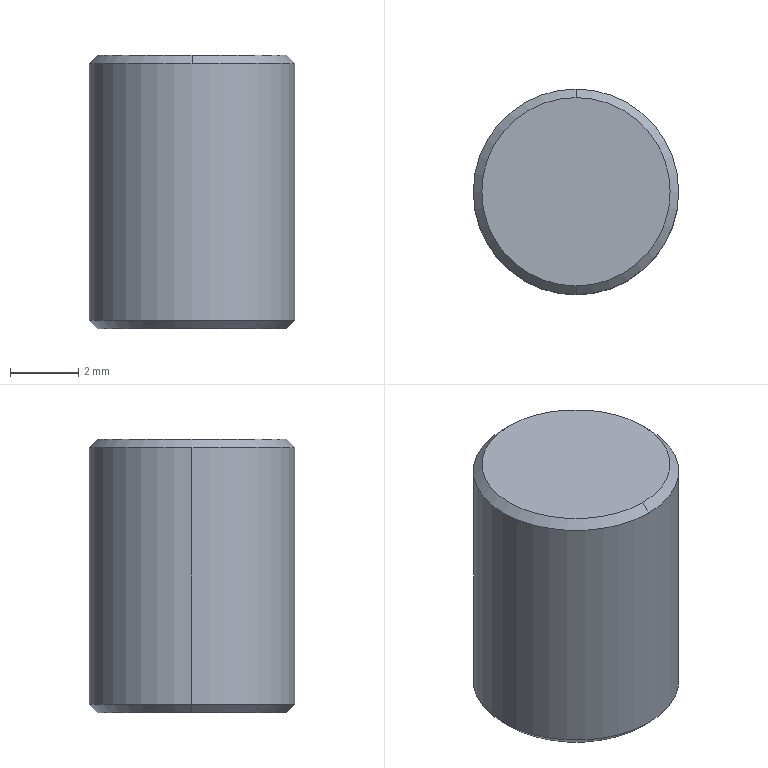Part | STEP file | CHOT TRUOT 6 LY | 1 solid | 8 faces | box 6 x 6 x 8 mm | volume 225.049 mm3 | cone 4 | cylinder 2 | plane 2 | commonest cylinder face diameters 6 x2
STEP:
#1=CARTESIAN_POINT('',(0.,0.,0.));
#2=DIRECTION('',(0.,0.,1.));
#3=DIRECTION('',(1.,0.,0.));
#4=AXIS2_PLACEMENT_3D('',#1,#2,#3);
#5=CARTESIAN_POINT('',(3.,0.,0.25));
#6=VERTEX_POINT('',#5);
#7=CARTESIAN_POINT('',(-3.,0.,0.25));
#8=VERTEX_POINT('',#7);
#9=CARTESIAN_POINT('',(0.,0.,0.25));
#10=DIRECTION('',(0.,0.,1.));
#11=DIRECTION('',(1.,0.,0.));
#12=AXIS2_PLACEMENT_3D('',#9,#10,#11);
#13=CIRCLE('',#12,3.);
#14=CARTESIAN_POINT('',(0.,0.,0.));
#15=DIRECTION('',(0.,0.,1.));
#16=DIRECTION('',(1.,0.,0.));
#17=AXIS2_PLACEMENT_3D('',#14,#15,#16);
#18=CYLINDRICAL_SURFACE('',#17,3.);
#19=CARTESIAN_POINT('',(0.,0.25));
#20=DIRECTION('',(1.,0.));
#21=VECTOR('',#20,1.);
#22=LINE('',#19,#21);
#23=(GEOMETRIC_REPRESENTATION_CONTEXT(2)PARAMETRIC_REPRESENTATION_CONTEXT()REPRESENTATION_CONTEXT('',''));
#24=DEFINITIONAL_REPRESENTATION('',(#22),#23);
#25=PCURVE('',#18,#24);
#26=CARTESIAN_POINT('',(0.,0.,0.25));
#27=DIRECTION('',(0.,0.,1.));
#28=DIRECTION('',(1.,0.,0.));
#29=AXIS2_PLACEMENT_3D('',#26,#27,#28);
#30=CONICAL_SURFACE('',#29,3.,0.7854);
#31=CARTESIAN_POINT('',(0.,0.));
#32=DIRECTION('',(1.,0.));
#33=VECTOR('',#32,1.);
#34=LINE('',#31,#33);
#35=(GEOMETRIC_REPRESENTATION_CONTEXT(2)PARAMETRIC_REPRESENTATION_CONTEXT()REPRESENTATION_CONTEXT('',''));
#36=DEFINITIONAL_REPRESENTATION('',(#34),#35);
#37=PCURVE('',#30,#36);
#38=SURFACE_CURVE('',#13,(#25,#37),.PCURVE_S1.);
#39=EDGE_CURVE('',#6,#8,#38,.T.);
#40=ORIENTED_EDGE('',*,*,#39,.T.);
#41=CARTESIAN_POINT('',(-3.,0.,7.75));
#42=VERTEX_POINT('',#41);
#43=CARTESIAN_POINT('',(-3.,0.,0.));
#44=DIRECTION('',(0.,0.,1.));
#45=VECTOR('',#44,1.);
#46=LINE('',#43,#45);
#47=CARTESIAN_POINT('',(3.142,0.));
#48=DIRECTION('',(0.,1.));
#49=VECTOR('',#48,1.);
#50=LINE('',#47,#49);
#51=(GEOMETRIC_REPRESENTATION_CONTEXT(2)PARAMETRIC_REPRESENTATION_CONTEXT()REPRESENTATION_CONTEXT('',''));
#52=DEFINITIONAL_REPRESENTATION('',(#50),#51);
#53=PCURVE('',#18,#52);
#54=CARTESIAN_POINT('',(0.,0.,0.));
#55=DIRECTION('',(0.,0.,1.));
#56=DIRECTION('',(1.,0.,0.));
#57=AXIS2_PLACEMENT_3D('',#54,#55,#56);
#58=CYLINDRICAL_SURFACE('',#57,3.);
#59=CARTESIAN_POINT('',(3.142,0.));
#60=DIRECTION('',(0.,1.));
#61=VECTOR('',#60,1.);
#62=LINE('',#59,#61);
#63=(GEOMETRIC_REPRESENTATION_CONTEXT(2)PARAMETRIC_REPRESENTATION_CONTEXT()REPRESENTATION_CONTEXT('',''));
#64=DEFINITIONAL_REPRESENTATION('',(#62),#63);
#65=PCURVE('',#58,#64);
#66=SURFACE_CURVE('',#46,(#53,#65),.PCURVE_S1.);
#67=EDGE_CURVE('',#8,#42,#66,.T.);
#68=ORIENTED_EDGE('',*,*,#67,.T.);
#69=CARTESIAN_POINT('',(0.,3.,7.75));
#70=VERTEX_POINT('',#69);
#71=CARTESIAN_POINT('',(0.,0.,7.75));
#72=DIRECTION('',(0.,0.,-1.));
#73=DIRECTION('',(1.,0.,0.));
#74=AXIS2_PLACEMENT_3D('',#71,#72,#73);
#75=CIRCLE('',#74,3.);
#76=CARTESIAN_POINT('',(6.283,7.75));
#77=DIRECTION('',(-1.,0.));
#78=VECTOR('',#77,1.);
#79=LINE('',#76,#78);
#80=(GEOMETRIC_REPRESENTATION_CONTEXT(2)PARAMETRIC_REPRESENTATION_CONTEXT()REPRESENTATION_CONTEXT('',''));
#81=DEFINITIONAL_REPRESENTATION('',(#79),#80);
#82=PCURVE('',#18,#81);
#83=CARTESIAN_POINT('',(0.,0.,7.75));
#84=DIRECTION('',(0.,0.,-1.));
#85=DIRECTION('',(0.,1.,0.));
#86=AXIS2_PLACEMENT_3D('',#83,#84,#85);
#87=CONICAL_SURFACE('',#86,3.,0.7854);
#88=CARTESIAN_POINT('',(1.571,0.));
#89=DIRECTION('',(1.,0.));
#90=VECTOR('',#89,1.);
#91=LINE('',#88,#90);
#92=(GEOMETRIC_REPRESENTATION_CONTEXT(2)PARAMETRIC_REPRESENTATION_CONTEXT()REPRESENTATION_CONTEXT('',''));
#93=DEFINITIONAL_REPRESENTATION('',(#91),#92);
#94=PCURVE('',#87,#93);
#95=SURFACE_CURVE('',#75,(#82,#94),.PCURVE_S1.);
#96=EDGE_CURVE('',#42,#70,#95,.T.);
#97=ORIENTED_EDGE('',*,*,#96,.T.);
#98=CARTESIAN_POINT('',(3.,0.,7.75));
#99=VERTEX_POINT('',#98);
#100=CARTESIAN_POINT('',(0.,0.,7.75));
#101=DIRECTION('',(0.,0.,-1.));
#102=DIRECTION('',(1.,0.,0.));
#103=AXIS2_PLACEMENT_3D('',#100,#101,#102);
#104=CIRCLE('',#103,3.);
#105=CARTESIAN_POINT('',(6.283,7.75));
#106=DIRECTION('',(-1.,0.));
#107=VECTOR('',#106,1.);
#108=LINE('',#105,#107);
#109=(GEOMETRIC_REPRESENTATION_CONTEXT(2)PARAMETRIC_REPRESENTATION_CONTEXT()REPRESENTATION_CONTEXT('',''));
#110=DEFINITIONAL_REPRESENTATION('',(#108),#109);
#111=PCURVE('',#18,#110);
#112=CARTESIAN_POINT('',(0.,0.,7.75));
#113=DIRECTION('',(0.,0.,-1.));
#114=DIRECTION('',(0.,1.,0.));
#115=AXIS2_PLACEMENT_3D('',#112,#113,#114);
#116=CONICAL_SURFACE('',#115,3.,0.7854);
#117=CARTESIAN_POINT('',(-4.712,0.));
#118=DIRECTION('',(1.,0.));
#119=VECTOR('',#118,1.);
#120=LINE('',#117,#119);
#121=(GEOMETRIC_REPRESENTATION_CONTEXT(2)PARAMETRIC_REPRESENTATION_CONTEXT()REPRESENTATION_CONTEXT('',''));
#122=DEFINITIONAL_REPRESENTATION('',(#120),#121);
#123=PCURVE('',#116,#122);
#124=SURFACE_CURVE('',#104,(#111,#123),.PCURVE_S1.);
#125=EDGE_CURVE('',#70,#99,#124,.T.);
#126=ORIENTED_EDGE('',*,*,#125,.T.);
#127=CARTESIAN_POINT('',(3.,0.,0.));
#128=DIRECTION('',(0.,0.,1.));
#129=VECTOR('',#128,1.);
#130=LINE('',#127,#129);
#131=CARTESIAN_POINT('',(0.,0.));
#132=DIRECTION('',(0.,1.));
#133=VECTOR('',#132,1.);
#134=LINE('',#131,#133);
#135=(GEOMETRIC_REPRESENTATION_CONTEXT(2)PARAMETRIC_REPRESENTATION_CONTEXT()REPRESENTATION_CONTEXT('',''));
#136=DEFINITIONAL_REPRESENTATION('',(#134),#135);
#137=PCURVE('',#18,#136);
#138=CARTESIAN_POINT('',(6.283,0.));
#139=DIRECTION('',(0.,1.));
#140=VECTOR('',#139,1.);
#141=LINE('',#138,#140);
#142=(GEOMETRIC_REPRESENTATION_CONTEXT(2)PARAMETRIC_REPRESENTATION_CONTEXT()REPRESENTATION_CONTEXT('',''));
#143=DEFINITIONAL_REPRESENTATION('',(#141),#142);
#144=PCURVE('',#58,#143);
#145=SURFACE_CURVE('',#130,(#137,#144),.PCURVE_S1.);
#146=EDGE_CURVE('',#6,#99,#145,.T.);
#147=ORIENTED_EDGE('',*,*,#146,.F.);
#148=EDGE_LOOP('',(#40,#68,#97,#126,#147));
#149=FACE_BOUND('',#148,.T.);
#150=ADVANCED_FACE('',(#149),#18,.T.);
#151=CARTESIAN_POINT('',(2.75,0.,0.));
#152=VERTEX_POINT('',#151);
#153=CARTESIAN_POINT('',(-2.75,0.,0.));
#154=VERTEX_POINT('',#153);
#155=CARTESIAN_POINT('',(0.,0.,0.));
#156=DIRECTION('',(0.,0.,1.));
#157=DIRECTION('',(1.,0.,0.));
#158=AXIS2_PLACEMENT_3D('',#155,#156,#157);
#159=CIRCLE('',#158,2.75);
#160=CARTESIAN_POINT('',(0.,-0.25));
#161=DIRECTION('',(1.,0.));
#162=VECTOR('',#161,1.);
#163=LINE('',#160,#162);
#164=(GEOMETRIC_REPRESENTATION_CONTEXT(2)PARAMETRIC_REPRESENTATION_CONTEXT()REPRESENTATION_CONTEXT('',''));
#165=DEFINITIONAL_REPRESENTATION('',(#163),#164);
#166=PCURVE('',#30,#165);
#167=CARTESIAN_POINT('',(0.,0.,0.));
#168=DIRECTION('',(0.,0.,-1.));
#169=DIRECTION('',(-1.,0.,0.));
#170=AXIS2_PLACEMENT_3D('',#167,#168,#169);
#171=PLANE('',#170);
#172=CARTESIAN_POINT('',(-2.75,0.));
#173=CARTESIAN_POINT('',(-2.75,4.763));
#174=CARTESIAN_POINT('',(1.375,2.382));
#175=CARTESIAN_POINT('',(5.5,0.));
#176=CARTESIAN_POINT('',(1.375,-2.382));
#177=CARTESIAN_POINT('',(-2.75,-4.763));
#178=CARTESIAN_POINT('',(-2.75,0.));
#179=(BOUNDED_CURVE()B_SPLINE_CURVE(2,(#172,#173,#174,#175,#176,#177,#178),.UNSPECIFIED.,.T.,.F.)B_SPLINE_CURVE_WITH_KNOTS((1,2,2,2,2,1),(-2.094,0.,2.094,4.189,6.283,8.378),.UNSPECIFIED.)CURVE()GEOMETRIC_REPRESENTATION_ITEM()RATIONAL_B_SPLINE_CURVE((1.,0.5,1.,0.5,1.,0.5,1.))REPRESENTATION_ITEM(''));
#180=(GEOMETRIC_REPRESENTATION_CONTEXT(2)PARAMETRIC_REPRESENTATION_CONTEXT()REPRESENTATION_CONTEXT('',''));
#181=DEFINITIONAL_REPRESENTATION('',(#179),#180);
#182=PCURVE('',#171,#181);
#183=SURFACE_CURVE('',#159,(#166,#182),.PCURVE_S1.);
#184=EDGE_CURVE('',#152,#154,#183,.T.);
#185=ORIENTED_EDGE('',*,*,#184,.T.);
#186=CARTESIAN_POINT('',(-3.,0.,0.25));
#187=DIRECTION('',(-0.7071,0.,0.7071));
#188=VECTOR('',#187,1.);
#189=LINE('',#186,#188);
#190=CARTESIAN_POINT('',(3.142,0.));
#191=DIRECTION('',(0.,1.));
#192=VECTOR('',#191,1.);
#193=LINE('',#190,#192);
#194=(GEOMETRIC_REPRESENTATION_CONTEXT(2)PARAMETRIC_REPRESENTATION_CONTEXT()REPRESENTATION_CONTEXT('',''));
#195=DEFINITIONAL_REPRESENTATION('',(#193),#194);
#196=PCURVE('',#30,#195);
#197=CARTESIAN_POINT('',(0.,0.,0.25));
#198=DIRECTION('',(0.,0.,1.));
#199=DIRECTION('',(1.,0.,0.));
#200=AXIS2_PLACEMENT_3D('',#197,#198,#199);
#201=CONICAL_SURFACE('',#200,3.,0.7854);
#202=CARTESIAN_POINT('',(3.142,0.));
#203=DIRECTION('',(0.,1.));
#204=VECTOR('',#203,1.);
#205=LINE('',#202,#204);
#206=(GEOMETRIC_REPRESENTATION_CONTEXT(2)PARAMETRIC_REPRESENTATION_CONTEXT()REPRESENTATION_CONTEXT('',''));
#207=DEFINITIONAL_REPRESENTATION('',(#205),#206);
#208=PCURVE('',#201,#207);
#209=SURFACE_CURVE('',#189,(#196,#208),.PCURVE_S1.);
#210=EDGE_CURVE('',#154,#8,#209,.T.);
#211=ORIENTED_EDGE('',*,*,#210,.T.);
#212=ORIENTED_EDGE('',*,*,#39,.F.);
#213=CARTESIAN_POINT('',(3.,0.,0.25));
#214=DIRECTION('',(0.7071,0.,0.7071));
#215=VECTOR('',#214,1.);
#216=LINE('',#213,#215);
#217=CARTESIAN_POINT('',(0.,0.));
#218=DIRECTION('',(0.,1.));
#219=VECTOR('',#218,1.);
#220=LINE('',#217,#219);
#221=(GEOMETRIC_REPRESENTATION_CONTEXT(2)PARAMETRIC_REPRESENTATION_CONTEXT()REPRESENTATION_CONTEXT('',''));
#222=DEFINITIONAL_REPRESENTATION('',(#220),#221);
#223=PCURVE('',#30,#222);
#224=CARTESIAN_POINT('',(6.283,0.));
#225=DIRECTION('',(0.,1.));
#226=VECTOR('',#225,1.);
#227=LINE('',#224,#226);
#228=(GEOMETRIC_REPRESENTATION_CONTEXT(2)PARAMETRIC_REPRESENTATION_CONTEXT()REPRESENTATION_CONTEXT('',''));
#229=DEFINITIONAL_REPRESENTATION('',(#227),#228);
#230=PCURVE('',#201,#229);
#231=SURFACE_CURVE('',#216,(#223,#230),.PCURVE_S1.);
#232=EDGE_CURVE('',#152,#6,#231,.T.);
#233=ORIENTED_EDGE('',*,*,#232,.F.);
#234=EDGE_LOOP('',(#185,#211,#212,#233));
#235=FACE_BOUND('',#234,.T.);
#236=ADVANCED_FACE('',(#235),#30,.T.);
#237=CARTESIAN_POINT('',(0.,2.75,8.));
#238=VERTEX_POINT('',#237);
#239=CARTESIAN_POINT('',(0.,-2.75,8.));
#240=VERTEX_POINT('',#239);
#241=CARTESIAN_POINT('',(0.,0.,8.));
#242=DIRECTION('',(0.,0.,-1.));
#243=DIRECTION('',(0.,1.,0.));
#244=AXIS2_PLACEMENT_3D('',#241,#242,#243);
#245=CIRCLE('',#244,2.75);
#246=CARTESIAN_POINT('',(0.,-0.25));
#247=DIRECTION('',(1.,0.));
#248=VECTOR('',#247,1.);
#249=LINE('',#246,#248);
#250=(GEOMETRIC_REPRESENTATION_CONTEXT(2)PARAMETRIC_REPRESENTATION_CONTEXT()REPRESENTATION_CONTEXT('',''));
#251=DEFINITIONAL_REPRESENTATION('',(#249),#250);
#252=PCURVE('',#116,#251);
#253=CARTESIAN_POINT('',(0.,0.,8.));
#254=DIRECTION('',(0.,0.,-1.));
#255=DIRECTION('',(-1.,0.,0.));
#256=AXIS2_PLACEMENT_3D('',#253,#254,#255);
#257=PLANE('',#256);
#258=CARTESIAN_POINT('',(0.,0.));
#259=DIRECTION('',(0.,1.));
#260=AXIS2_PLACEMENT_2D('',#258,#259);
#261=CIRCLE('',#260,2.75);
#262=(GEOMETRIC_REPRESENTATION_CONTEXT(2)PARAMETRIC_REPRESENTATION_CONTEXT()REPRESENTATION_CONTEXT('',''));
#263=DEFINITIONAL_REPRESENTATION('',(#261),#262);
#264=PCURVE('',#257,#263);
#265=SURFACE_CURVE('',#245,(#252,#264),.PCURVE_S1.);
#266=EDGE_CURVE('',#238,#240,#265,.T.);
#267=ORIENTED_EDGE('',*,*,#266,.T.);
#268=CARTESIAN_POINT('',(0.,-3.,7.75));
#269=VERTEX_POINT('',#268);
#270=CARTESIAN_POINT('',(0.,-3.,7.75));
#271=DIRECTION('',(0.,-0.7071,-0.7071));
#272=VECTOR('',#271,1.);
#273=LINE('',#270,#272);
#274=CARTESIAN_POINT('',(3.142,0.));
#275=DIRECTION('',(0.,1.));
#276=VECTOR('',#275,1.);
#277=LINE('',#274,#276);
#278=(GEOMETRIC_REPRESENTATION_CONTEXT(2)PARAMETRIC_REPRESENTATION_CONTEXT()REPRESENTATION_CONTEXT('',''));
#279=DEFINITIONAL_REPRESENTATION('',(#277),#278);
#280=PCURVE('',#116,#279);
#281=CARTESIAN_POINT('',(3.142,0.));
#282=DIRECTION('',(0.,1.));
#283=VECTOR('',#282,1.);
#284=LINE('',#281,#283);
#285=(GEOMETRIC_REPRESENTATION_CONTEXT(2)PARAMETRIC_REPRESENTATION_CONTEXT()REPRESENTATION_CONTEXT('',''));
#286=DEFINITIONAL_REPRESENTATION('',(#284),#285);
#287=PCURVE('',#87,#286);
#288=SURFACE_CURVE('',#273,(#280,#287),.PCURVE_S1.);
#289=EDGE_CURVE('',#240,#269,#288,.T.);
#290=ORIENTED_EDGE('',*,*,#289,.T.);
#291=CARTESIAN_POINT('',(0.,0.,7.75));
#292=DIRECTION('',(0.,0.,-1.));
#293=DIRECTION('',(1.,0.,0.));
#294=AXIS2_PLACEMENT_3D('',#291,#292,#293);
#295=CIRCLE('',#294,3.);
#296=CARTESIAN_POINT('',(1.571,0.));
#297=DIRECTION('',(1.,0.));
#298=VECTOR('',#297,1.);
#299=LINE('',#296,#298);
#300=(GEOMETRIC_REPRESENTATION_CONTEXT(2)PARAMETRIC_REPRESENTATION_CONTEXT()REPRESENTATION_CONTEXT('',''));
#301=DEFINITIONAL_REPRESENTATION('',(#299),#300);
#302=PCURVE('',#116,#301);
#303=CARTESIAN_POINT('',(6.283,7.75));
#304=DIRECTION('',(-1.,0.));
#305=VECTOR('',#304,1.);
#306=LINE('',#303,#305);
#307=(GEOMETRIC_REPRESENTATION_CONTEXT(2)PARAMETRIC_REPRESENTATION_CONTEXT()REPRESENTATION_CONTEXT('',''));
#308=DEFINITIONAL_REPRESENTATION('',(#306),#307);
#309=PCURVE('',#58,#308);
#310=SURFACE_CURVE('',#295,(#302,#309),.PCURVE_S1.);
#311=EDGE_CURVE('',#99,#269,#310,.T.);
#312=ORIENTED_EDGE('',*,*,#311,.F.);
#313=ORIENTED_EDGE('',*,*,#125,.F.);
#314=CARTESIAN_POINT('',(0.,3.,7.75));
#315=DIRECTION('',(0.,0.7071,-0.7071));
#316=VECTOR('',#315,1.);
#317=LINE('',#314,#316);
#318=CARTESIAN_POINT('',(0.,0.));
#319=DIRECTION('',(0.,1.));
#320=VECTOR('',#319,1.);
#321=LINE('',#318,#320);
#322=(GEOMETRIC_REPRESENTATION_CONTEXT(2)PARAMETRIC_REPRESENTATION_CONTEXT()REPRESENTATION_CONTEXT('',''));
#323=DEFINITIONAL_REPRESENTATION('',(#321),#322);
#324=PCURVE('',#116,#323);
#325=CARTESIAN_POINT('',(6.283,0.));
#326=DIRECTION('',(0.,1.));
#327=VECTOR('',#326,1.);
#328=LINE('',#325,#327);
#329=(GEOMETRIC_REPRESENTATION_CONTEXT(2)PARAMETRIC_REPRESENTATION_CONTEXT()REPRESENTATION_CONTEXT('',''));
#330=DEFINITIONAL_REPRESENTATION('',(#328),#329);
#331=PCURVE('',#87,#330);
#332=SURFACE_CURVE('',#317,(#324,#331),.PCURVE_S1.);
#333=EDGE_CURVE('',#238,#70,#332,.T.);
#334=ORIENTED_EDGE('',*,*,#333,.F.);
#335=EDGE_LOOP('',(#267,#290,#312,#313,#334));
#336=FACE_BOUND('',#335,.T.);
#337=ADVANCED_FACE('',(#336),#116,.T.);
#338=ORIENTED_EDGE('',*,*,#67,.F.);
#339=CARTESIAN_POINT('',(0.,0.,0.25));
#340=DIRECTION('',(0.,0.,1.));
#341=DIRECTION('',(1.,0.,0.));
#342=AXIS2_PLACEMENT_3D('',#339,#340,#341);
#343=CIRCLE('',#342,3.);
#344=CARTESIAN_POINT('',(0.,0.25));
#345=DIRECTION('',(1.,0.));
#346=VECTOR('',#345,1.);
#347=LINE('',#344,#346);
#348=(GEOMETRIC_REPRESENTATION_CONTEXT(2)PARAMETRIC_REPRESENTATION_CONTEXT()REPRESENTATION_CONTEXT('',''));
#349=DEFINITIONAL_REPRESENTATION('',(#347),#348);
#350=PCURVE('',#58,#349);
#351=CARTESIAN_POINT('',(0.,0.));
#352=DIRECTION('',(1.,0.));
#353=VECTOR('',#352,1.);
#354=LINE('',#351,#353);
#355=(GEOMETRIC_REPRESENTATION_CONTEXT(2)PARAMETRIC_REPRESENTATION_CONTEXT()REPRESENTATION_CONTEXT('',''));
#356=DEFINITIONAL_REPRESENTATION('',(#354),#355);
#357=PCURVE('',#201,#356);
#358=SURFACE_CURVE('',#343,(#350,#357),.PCURVE_S1.);
#359=EDGE_CURVE('',#8,#6,#358,.T.);
#360=ORIENTED_EDGE('',*,*,#359,.T.);
#361=ORIENTED_EDGE('',*,*,#146,.T.);
#362=ORIENTED_EDGE('',*,*,#311,.T.);
#363=CARTESIAN_POINT('',(0.,0.,7.75));
#364=DIRECTION('',(0.,0.,-1.));
#365=DIRECTION('',(1.,0.,0.));
#366=AXIS2_PLACEMENT_3D('',#363,#364,#365);
#367=CIRCLE('',#366,3.);
#368=CARTESIAN_POINT('',(6.283,7.75));
#369=DIRECTION('',(-1.,0.));
#370=VECTOR('',#369,1.);
#371=LINE('',#368,#370);
#372=(GEOMETRIC_REPRESENTATION_CONTEXT(2)PARAMETRIC_REPRESENTATION_CONTEXT()REPRESENTATION_CONTEXT('',''));
#373=DEFINITIONAL_REPRESENTATION('',(#371),#372);
#374=PCURVE('',#58,#373);
#375=CARTESIAN_POINT('',(1.571,0.));
#376=DIRECTION('',(1.,0.));
#377=VECTOR('',#376,1.);
#378=LINE('',#375,#377);
#379=(GEOMETRIC_REPRESENTATION_CONTEXT(2)PARAMETRIC_REPRESENTATION_CONTEXT()REPRESENTATION_CONTEXT('',''));
#380=DEFINITIONAL_REPRESENTATION('',(#378),#379);
#381=PCURVE('',#87,#380);
#382=SURFACE_CURVE('',#367,(#374,#381),.PCURVE_S1.);
#383=EDGE_CURVE('',#269,#42,#382,.T.);
#384=ORIENTED_EDGE('',*,*,#383,.T.);
#385=EDGE_LOOP('',(#338,#360,#361,#362,#384));
#386=FACE_BOUND('',#385,.T.);
#387=ADVANCED_FACE('',(#386),#58,.T.);
#388=ORIENTED_EDGE('',*,*,#210,.F.);
#389=CARTESIAN_POINT('',(0.,0.,0.));
#390=DIRECTION('',(0.,0.,1.));
#391=DIRECTION('',(1.,0.,0.));
#392=AXIS2_PLACEMENT_3D('',#389,#390,#391);
#393=CIRCLE('',#392,2.75);
#394=CARTESIAN_POINT('',(0.,-0.25));
#395=DIRECTION('',(1.,0.));
#396=VECTOR('',#395,1.);
#397=LINE('',#394,#396);
#398=(GEOMETRIC_REPRESENTATION_CONTEXT(2)PARAMETRIC_REPRESENTATION_CONTEXT()REPRESENTATION_CONTEXT('',''));
#399=DEFINITIONAL_REPRESENTATION('',(#397),#398);
#400=PCURVE('',#201,#399);
#401=CARTESIAN_POINT('',(-2.75,0.));
#402=CARTESIAN_POINT('',(-2.75,4.763));
#403=CARTESIAN_POINT('',(1.375,2.382));
#404=CARTESIAN_POINT('',(5.5,0.));
#405=CARTESIAN_POINT('',(1.375,-2.382));
#406=CARTESIAN_POINT('',(-2.75,-4.763));
#407=CARTESIAN_POINT('',(-2.75,0.));
#408=(BOUNDED_CURVE()B_SPLINE_CURVE(2,(#401,#402,#403,#404,#405,#406,#407),.UNSPECIFIED.,.T.,.F.)B_SPLINE_CURVE_WITH_KNOTS((1,2,2,2,2,1),(-2.094,0.,2.094,4.189,6.283,8.378),.UNSPECIFIED.)CURVE()GEOMETRIC_REPRESENTATION_ITEM()RATIONAL_B_SPLINE_CURVE((1.,0.5,1.,0.5,1.,0.5,1.))REPRESENTATION_ITEM(''));
#409=(GEOMETRIC_REPRESENTATION_CONTEXT(2)PARAMETRIC_REPRESENTATION_CONTEXT()REPRESENTATION_CONTEXT('',''));
#410=DEFINITIONAL_REPRESENTATION('',(#408),#409);
#411=PCURVE('',#171,#410);
#412=SURFACE_CURVE('',#393,(#400,#411),.PCURVE_S1.);
#413=EDGE_CURVE('',#154,#152,#412,.T.);
#414=ORIENTED_EDGE('',*,*,#413,.T.);
#415=ORIENTED_EDGE('',*,*,#232,.T.);
#416=ORIENTED_EDGE('',*,*,#359,.F.);
#417=EDGE_LOOP('',(#388,#414,#415,#416));
#418=FACE_BOUND('',#417,.T.);
#419=ADVANCED_FACE('',(#418),#201,.T.);
#420=ORIENTED_EDGE('',*,*,#289,.F.);
#421=CARTESIAN_POINT('',(0.,0.,8.));
#422=DIRECTION('',(0.,0.,-1.));
#423=DIRECTION('',(0.,1.,0.));
#424=AXIS2_PLACEMENT_3D('',#421,#422,#423);
#425=CIRCLE('',#424,2.75);
#426=CARTESIAN_POINT('',(0.,-0.25));
#427=DIRECTION('',(1.,0.));
#428=VECTOR('',#427,1.);
#429=LINE('',#426,#428);
#430=(GEOMETRIC_REPRESENTATION_CONTEXT(2)PARAMETRIC_REPRESENTATION_CONTEXT()REPRESENTATION_CONTEXT('',''));
#431=DEFINITIONAL_REPRESENTATION('',(#429),#430);
#432=PCURVE('',#87,#431);
#433=CARTESIAN_POINT('',(0.,0.));
#434=DIRECTION('',(0.,1.));
#435=AXIS2_PLACEMENT_2D('',#433,#434);
#436=CIRCLE('',#435,2.75);
#437=(GEOMETRIC_REPRESENTATION_CONTEXT(2)PARAMETRIC_REPRESENTATION_CONTEXT()REPRESENTATION_CONTEXT('',''));
#438=DEFINITIONAL_REPRESENTATION('',(#436),#437);
#439=PCURVE('',#257,#438);
#440=SURFACE_CURVE('',#425,(#432,#439),.PCURVE_S1.);
#441=EDGE_CURVE('',#240,#238,#440,.T.);
#442=ORIENTED_EDGE('',*,*,#441,.T.);
#443=ORIENTED_EDGE('',*,*,#333,.T.);
#444=ORIENTED_EDGE('',*,*,#96,.F.);
#445=ORIENTED_EDGE('',*,*,#383,.F.);
#446=EDGE_LOOP('',(#420,#442,#443,#444,#445));
#447=FACE_BOUND('',#446,.T.);
#448=ADVANCED_FACE('',(#447),#87,.T.);
#449=ORIENTED_EDGE('',*,*,#184,.F.);
#450=ORIENTED_EDGE('',*,*,#413,.F.);
#451=EDGE_LOOP('',(#449,#450));
#452=FACE_BOUND('',#451,.T.);
#453=ADVANCED_FACE('',(#452),#171,.T.);
#454=ORIENTED_EDGE('',*,*,#266,.F.);
#455=ORIENTED_EDGE('',*,*,#441,.F.);
#456=EDGE_LOOP('',(#454,#455));
#457=FACE_BOUND('',#456,.T.);
#458=ADVANCED_FACE('',(#457),#257,.F.);
#459=CLOSED_SHELL('',(#150,#236,#337,#387,#419,#448,#453,#458));
#460=MANIFOLD_SOLID_BREP('',#459);
#461=(LENGTH_UNIT()NAMED_UNIT(*)SI_UNIT(.MILLI.,.METRE.));
#462=UNCERTAINTY_MEASURE_WITH_UNIT(LENGTH_MEASURE(0.0000001),#461,'','');
#463=(NAMED_UNIT(*)PLANE_ANGLE_UNIT()SI_UNIT($,.RADIAN.));
#464=(NAMED_UNIT(*)SI_UNIT($,.STERADIAN.)SOLID_ANGLE_UNIT());
#465=(GEOMETRIC_REPRESENTATION_CONTEXT(3)GLOBAL_UNCERTAINTY_ASSIGNED_CONTEXT((#462))GLOBAL_UNIT_ASSIGNED_CONTEXT((#461,#463,#464))REPRESENTATION_CONTEXT('',''));
#466=ADVANCED_BREP_SHAPE_REPRESENTATION('',(#4,#460),#465);